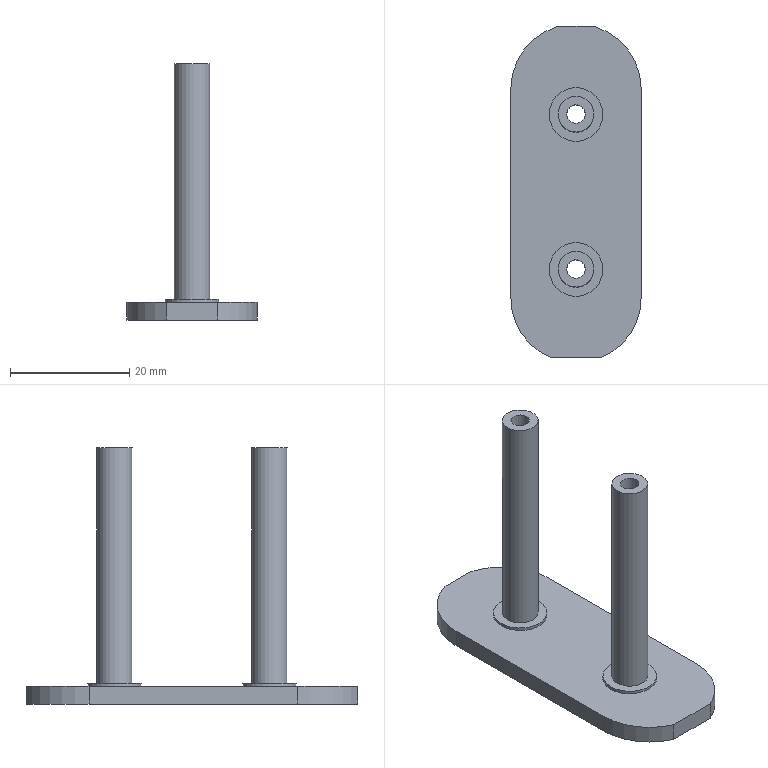Part | STEP file | Wytnij-wyci_gni_cie1 | 1 solid | 20 faces | box 21.875 x 55.54 x 43 mm | volume 5051 mm3 | cylinder 10 | plane 10 | commonest cylinder face diameters 21.875 x4 3.1 x2 6 x2 9 x2
STEP:
#1=CARTESIAN_POINT('',(0.,0.,0.));
#2=DIRECTION('',(0.,0.,1.));
#3=DIRECTION('',(1.,0.,0.));
#4=AXIS2_PLACEMENT_3D('',#1,#2,#3);
#5=CARTESIAN_POINT('',(-37.194,75.138,-134.798));
#6=VERTEX_POINT('',#5);
#7=CARTESIAN_POINT('',(-38.744,75.138,-134.798));
#8=DIRECTION('',(0.,0.,-1.));
#9=DIRECTION('',(1.,0.,0.));
#10=AXIS2_PLACEMENT_3D('',#7,#8,#9);
#11=CIRCLE('',#10,1.55);
#12=CARTESIAN_POINT('',(-38.744,75.138,-134.798));
#13=DIRECTION('',(0.,0.,1.));
#14=DIRECTION('',(1.,0.,0.));
#15=AXIS2_PLACEMENT_3D('',#12,#13,#14);
#16=CYLINDRICAL_SURFACE('',#15,1.55);
#17=CARTESIAN_POINT('',(6.283,0.));
#18=DIRECTION('',(-1.,0.));
#19=VECTOR('',#18,1.);
#20=LINE('',#17,#19);
#21=(GEOMETRIC_REPRESENTATION_CONTEXT(2)PARAMETRIC_REPRESENTATION_CONTEXT()REPRESENTATION_CONTEXT('',''));
#22=DEFINITIONAL_REPRESENTATION('',(#20),#21);
#23=PCURVE('',#16,#22);
#24=CARTESIAN_POINT('',(-38.744,88.138,-134.798));
#25=DIRECTION('',(0.,0.,1.));
#26=DIRECTION('',(1.,0.,0.));
#27=AXIS2_PLACEMENT_3D('',#24,#25,#26);
#28=PLANE('',#27);
#29=CARTESIAN_POINT('',(1.55,-13.));
#30=CARTESIAN_POINT('',(1.55,-15.685));
#31=CARTESIAN_POINT('',(-0.775,-14.342));
#32=CARTESIAN_POINT('',(-3.1,-13.));
#33=CARTESIAN_POINT('',(-0.775,-11.658));
#34=CARTESIAN_POINT('',(1.55,-10.315));
#35=CARTESIAN_POINT('',(1.55,-13.));
#36=(BOUNDED_CURVE()B_SPLINE_CURVE(2,(#29,#30,#31,#32,#33,#34,#35),.UNSPECIFIED.,.T.,.F.)B_SPLINE_CURVE_WITH_KNOTS((1,2,2,2,2,1),(-2.094,0.,2.094,4.189,6.283,8.378),.UNSPECIFIED.)CURVE()GEOMETRIC_REPRESENTATION_ITEM()RATIONAL_B_SPLINE_CURVE((1.,0.5,1.,0.5,1.,0.5,1.))REPRESENTATION_ITEM(''));
#37=(GEOMETRIC_REPRESENTATION_CONTEXT(2)PARAMETRIC_REPRESENTATION_CONTEXT()REPRESENTATION_CONTEXT('',''));
#38=DEFINITIONAL_REPRESENTATION('',(#36),#37);
#39=PCURVE('',#28,#38);
#40=SURFACE_CURVE('',#11,(#23,#39),.PCURVE_S1.);
#41=EDGE_CURVE('',#6,#6,#40,.T.);
#42=ORIENTED_EDGE('',*,*,#41,.F.);
#43=CARTESIAN_POINT('',(-37.194,75.138,-91.798));
#44=VERTEX_POINT('',#43);
#45=CARTESIAN_POINT('',(-37.194,75.138,-91.798));
#46=DIRECTION('',(0.,0.,-1.));
#47=VECTOR('',#46,1.);
#48=LINE('',#45,#47);
#49=CARTESIAN_POINT('',(6.283,43.));
#50=DIRECTION('',(0.,-1.));
#51=VECTOR('',#50,1.);
#52=LINE('',#49,#51);
#53=(GEOMETRIC_REPRESENTATION_CONTEXT(2)PARAMETRIC_REPRESENTATION_CONTEXT()REPRESENTATION_CONTEXT('',''));
#54=DEFINITIONAL_REPRESENTATION('',(#52),#53);
#55=PCURVE('',#16,#54);
#56=CARTESIAN_POINT('',(0.,43.));
#57=DIRECTION('',(0.,-1.));
#58=VECTOR('',#57,1.);
#59=LINE('',#56,#58);
#60=(GEOMETRIC_REPRESENTATION_CONTEXT(2)PARAMETRIC_REPRESENTATION_CONTEXT()REPRESENTATION_CONTEXT('',''));
#61=DEFINITIONAL_REPRESENTATION('',(#59),#60);
#62=PCURVE('',#16,#61);
#63=SEAM_CURVE('',#48,(#55,#62),.PCURVE_S1.);
#64=EDGE_CURVE('',#44,#6,#63,.T.);
#65=ORIENTED_EDGE('',*,*,#64,.F.);
#66=CARTESIAN_POINT('',(-38.744,75.138,-91.798));
#67=DIRECTION('',(0.,0.,-1.));
#68=DIRECTION('',(1.,0.,0.));
#69=AXIS2_PLACEMENT_3D('',#66,#67,#68);
#70=CIRCLE('',#69,1.55);
#71=CARTESIAN_POINT('',(6.283,43.));
#72=DIRECTION('',(-1.,0.));
#73=VECTOR('',#72,1.);
#74=LINE('',#71,#73);
#75=(GEOMETRIC_REPRESENTATION_CONTEXT(2)PARAMETRIC_REPRESENTATION_CONTEXT()REPRESENTATION_CONTEXT('',''));
#76=DEFINITIONAL_REPRESENTATION('',(#74),#75);
#77=PCURVE('',#16,#76);
#78=CARTESIAN_POINT('',(-38.744,75.138,-91.798));
#79=DIRECTION('',(0.,0.,1.));
#80=DIRECTION('',(1.,0.,0.));
#81=AXIS2_PLACEMENT_3D('',#78,#79,#80);
#82=PLANE('',#81);
#83=CARTESIAN_POINT('',(1.55,0.));
#84=CARTESIAN_POINT('',(1.55,-2.685));
#85=CARTESIAN_POINT('',(-0.775,-1.342));
#86=CARTESIAN_POINT('',(-3.1,0.));
#87=CARTESIAN_POINT('',(-0.775,1.342));
#88=CARTESIAN_POINT('',(1.55,2.685));
#89=CARTESIAN_POINT('',(1.55,0.));
#90=(BOUNDED_CURVE()B_SPLINE_CURVE(2,(#83,#84,#85,#86,#87,#88,#89),.UNSPECIFIED.,.T.,.F.)B_SPLINE_CURVE_WITH_KNOTS((1,2,2,2,2,1),(-2.094,0.,2.094,4.189,6.283,8.378),.UNSPECIFIED.)CURVE()GEOMETRIC_REPRESENTATION_ITEM()RATIONAL_B_SPLINE_CURVE((1.,0.5,1.,0.5,1.,0.5,1.))REPRESENTATION_ITEM(''));
#91=(GEOMETRIC_REPRESENTATION_CONTEXT(2)PARAMETRIC_REPRESENTATION_CONTEXT()REPRESENTATION_CONTEXT('',''));
#92=DEFINITIONAL_REPRESENTATION('',(#90),#91);
#93=PCURVE('',#82,#92);
#94=SURFACE_CURVE('',#70,(#77,#93),.PCURVE_S1.);
#95=EDGE_CURVE('',#44,#44,#94,.T.);
#96=ORIENTED_EDGE('',*,*,#95,.T.);
#97=ORIENTED_EDGE('',*,*,#64,.T.);
#98=EDGE_LOOP('',(#42,#65,#96,#97));
#99=FACE_BOUND('',#98,.F.);
#100=ADVANCED_FACE('',(#99),#16,.F.);
#101=CARTESIAN_POINT('',(-37.194,101.138,-134.798));
#102=VERTEX_POINT('',#101);
#103=CARTESIAN_POINT('',(-38.744,101.138,-134.798));
#104=DIRECTION('',(0.,0.,-1.));
#105=DIRECTION('',(1.,0.,0.));
#106=AXIS2_PLACEMENT_3D('',#103,#104,#105);
#107=CIRCLE('',#106,1.55);
#108=CARTESIAN_POINT('',(-38.744,101.138,-134.798));
#109=DIRECTION('',(0.,0.,1.));
#110=DIRECTION('',(1.,0.,0.));
#111=AXIS2_PLACEMENT_3D('',#108,#109,#110);
#112=CYLINDRICAL_SURFACE('',#111,1.55);
#113=CARTESIAN_POINT('',(6.283,0.));
#114=DIRECTION('',(-1.,0.));
#115=VECTOR('',#114,1.);
#116=LINE('',#113,#115);
#117=(GEOMETRIC_REPRESENTATION_CONTEXT(2)PARAMETRIC_REPRESENTATION_CONTEXT()REPRESENTATION_CONTEXT('',''));
#118=DEFINITIONAL_REPRESENTATION('',(#116),#117);
#119=PCURVE('',#112,#118);
#120=CARTESIAN_POINT('',(1.55,13.));
#121=CARTESIAN_POINT('',(1.55,10.315));
#122=CARTESIAN_POINT('',(-0.775,11.658));
#123=CARTESIAN_POINT('',(-3.1,13.));
#124=CARTESIAN_POINT('',(-0.775,14.342));
#125=CARTESIAN_POINT('',(1.55,15.685));
#126=CARTESIAN_POINT('',(1.55,13.));
#127=(BOUNDED_CURVE()B_SPLINE_CURVE(2,(#120,#121,#122,#123,#124,#125,#126),.UNSPECIFIED.,.T.,.F.)B_SPLINE_CURVE_WITH_KNOTS((1,2,2,2,2,1),(-2.094,0.,2.094,4.189,6.283,8.378),.UNSPECIFIED.)CURVE()GEOMETRIC_REPRESENTATION_ITEM()RATIONAL_B_SPLINE_CURVE((1.,0.5,1.,0.5,1.,0.5,1.))REPRESENTATION_ITEM(''));
#128=(GEOMETRIC_REPRESENTATION_CONTEXT(2)PARAMETRIC_REPRESENTATION_CONTEXT()REPRESENTATION_CONTEXT('',''));
#129=DEFINITIONAL_REPRESENTATION('',(#127),#128);
#130=PCURVE('',#28,#129);
#131=SURFACE_CURVE('',#107,(#119,#130),.PCURVE_S1.);
#132=EDGE_CURVE('',#102,#102,#131,.T.);
#133=ORIENTED_EDGE('',*,*,#132,.F.);
#134=CARTESIAN_POINT('',(-37.194,101.138,-91.798));
#135=VERTEX_POINT('',#134);
#136=CARTESIAN_POINT('',(-37.194,101.138,-91.798));
#137=DIRECTION('',(0.,0.,-1.));
#138=VECTOR('',#137,1.);
#139=LINE('',#136,#138);
#140=CARTESIAN_POINT('',(6.283,43.));
#141=DIRECTION('',(0.,-1.));
#142=VECTOR('',#141,1.);
#143=LINE('',#140,#142);
#144=(GEOMETRIC_REPRESENTATION_CONTEXT(2)PARAMETRIC_REPRESENTATION_CONTEXT()REPRESENTATION_CONTEXT('',''));
#145=DEFINITIONAL_REPRESENTATION('',(#143),#144);
#146=PCURVE('',#112,#145);
#147=CARTESIAN_POINT('',(0.,43.));
#148=DIRECTION('',(0.,-1.));
#149=VECTOR('',#148,1.);
#150=LINE('',#147,#149);
#151=(GEOMETRIC_REPRESENTATION_CONTEXT(2)PARAMETRIC_REPRESENTATION_CONTEXT()REPRESENTATION_CONTEXT('',''));
#152=DEFINITIONAL_REPRESENTATION('',(#150),#151);
#153=PCURVE('',#112,#152);
#154=SEAM_CURVE('',#139,(#146,#153),.PCURVE_S1.);
#155=EDGE_CURVE('',#135,#102,#154,.T.);
#156=ORIENTED_EDGE('',*,*,#155,.F.);
#157=CARTESIAN_POINT('',(-38.744,101.138,-91.798));
#158=DIRECTION('',(0.,0.,-1.));
#159=DIRECTION('',(1.,0.,0.));
#160=AXIS2_PLACEMENT_3D('',#157,#158,#159);
#161=CIRCLE('',#160,1.55);
#162=CARTESIAN_POINT('',(6.283,43.));
#163=DIRECTION('',(-1.,0.));
#164=VECTOR('',#163,1.);
#165=LINE('',#162,#164);
#166=(GEOMETRIC_REPRESENTATION_CONTEXT(2)PARAMETRIC_REPRESENTATION_CONTEXT()REPRESENTATION_CONTEXT('',''));
#167=DEFINITIONAL_REPRESENTATION('',(#165),#166);
#168=PCURVE('',#112,#167);
#169=CARTESIAN_POINT('',(-38.744,101.138,-91.798));
#170=DIRECTION('',(0.,0.,1.));
#171=DIRECTION('',(1.,0.,0.));
#172=AXIS2_PLACEMENT_3D('',#169,#170,#171);
#173=PLANE('',#172);
#174=CARTESIAN_POINT('',(1.55,0.));
#175=CARTESIAN_POINT('',(1.55,-2.685));
#176=CARTESIAN_POINT('',(-0.775,-1.342));
#177=CARTESIAN_POINT('',(-3.1,0.));
#178=CARTESIAN_POINT('',(-0.775,1.342));
#179=CARTESIAN_POINT('',(1.55,2.685));
#180=CARTESIAN_POINT('',(1.55,0.));
#181=(BOUNDED_CURVE()B_SPLINE_CURVE(2,(#174,#175,#176,#177,#178,#179,#180),.UNSPECIFIED.,.T.,.F.)B_SPLINE_CURVE_WITH_KNOTS((1,2,2,2,2,1),(-2.094,0.,2.094,4.189,6.283,8.378),.UNSPECIFIED.)CURVE()GEOMETRIC_REPRESENTATION_ITEM()RATIONAL_B_SPLINE_CURVE((1.,0.5,1.,0.5,1.,0.5,1.))REPRESENTATION_ITEM(''));
#182=(GEOMETRIC_REPRESENTATION_CONTEXT(2)PARAMETRIC_REPRESENTATION_CONTEXT()REPRESENTATION_CONTEXT('',''));
#183=DEFINITIONAL_REPRESENTATION('',(#181),#182);
#184=PCURVE('',#173,#183);
#185=SURFACE_CURVE('',#161,(#168,#184),.PCURVE_S1.);
#186=EDGE_CURVE('',#135,#135,#185,.T.);
#187=ORIENTED_EDGE('',*,*,#186,.T.);
#188=ORIENTED_EDGE('',*,*,#155,.T.);
#189=EDGE_LOOP('',(#133,#156,#187,#188));
#190=FACE_BOUND('',#189,.F.);
#191=ADVANCED_FACE('',(#190),#112,.F.);
#192=CARTESIAN_POINT('',(-41.744,75.138,-131.298));
#193=VERTEX_POINT('',#192);
#194=CARTESIAN_POINT('',(-41.744,75.138,-91.798));
#195=VERTEX_POINT('',#194);
#196=CARTESIAN_POINT('',(-41.744,75.138,-131.298));
#197=DIRECTION('',(0.,0.,1.));
#198=VECTOR('',#197,1.);
#199=LINE('',#196,#198);
#200=CARTESIAN_POINT('',(-38.744,75.138,-91.798));
#201=DIRECTION('',(0.,0.,-1.));
#202=DIRECTION('',(-1.,0.,0.));
#203=AXIS2_PLACEMENT_3D('',#200,#201,#202);
#204=CYLINDRICAL_SURFACE('',#203,3.);
#205=CARTESIAN_POINT('',(0.,39.5));
#206=DIRECTION('',(0.,-1.));
#207=VECTOR('',#206,1.);
#208=LINE('',#205,#207);
#209=(GEOMETRIC_REPRESENTATION_CONTEXT(2)PARAMETRIC_REPRESENTATION_CONTEXT()REPRESENTATION_CONTEXT('',''));
#210=DEFINITIONAL_REPRESENTATION('',(#208),#209);
#211=PCURVE('',#204,#210);
#212=CARTESIAN_POINT('',(6.283,39.5));
#213=DIRECTION('',(0.,-1.));
#214=VECTOR('',#213,1.);
#215=LINE('',#212,#214);
#216=(GEOMETRIC_REPRESENTATION_CONTEXT(2)PARAMETRIC_REPRESENTATION_CONTEXT()REPRESENTATION_CONTEXT('',''));
#217=DEFINITIONAL_REPRESENTATION('',(#215),#216);
#218=PCURVE('',#204,#217);
#219=SEAM_CURVE('',#199,(#211,#218),.PCURVE_S1.);
#220=EDGE_CURVE('',#193,#195,#219,.T.);
#221=ORIENTED_EDGE('',*,*,#220,.T.);
#222=CARTESIAN_POINT('',(-38.744,75.138,-91.798));
#223=DIRECTION('',(0.,0.,1.));
#224=DIRECTION('',(-1.,0.,0.));
#225=AXIS2_PLACEMENT_3D('',#222,#223,#224);
#226=CIRCLE('',#225,3.);
#227=CARTESIAN_POINT('',(6.283,0.));
#228=DIRECTION('',(-1.,0.));
#229=VECTOR('',#228,1.);
#230=LINE('',#227,#229);
#231=(GEOMETRIC_REPRESENTATION_CONTEXT(2)PARAMETRIC_REPRESENTATION_CONTEXT()REPRESENTATION_CONTEXT('',''));
#232=DEFINITIONAL_REPRESENTATION('',(#230),#231);
#233=PCURVE('',#204,#232);
#234=CARTESIAN_POINT('',(0.,0.));
#235=DIRECTION('',(-1.,0.));
#236=AXIS2_PLACEMENT_2D('',#234,#235);
#237=CIRCLE('',#236,3.);
#238=(GEOMETRIC_REPRESENTATION_CONTEXT(2)PARAMETRIC_REPRESENTATION_CONTEXT()REPRESENTATION_CONTEXT('',''));
#239=DEFINITIONAL_REPRESENTATION('',(#237),#238);
#240=PCURVE('',#82,#239);
#241=SURFACE_CURVE('',#226,(#233,#240),.PCURVE_S1.);
#242=EDGE_CURVE('',#195,#195,#241,.T.);
#243=ORIENTED_EDGE('',*,*,#242,.F.);
#244=ORIENTED_EDGE('',*,*,#220,.F.);
#245=CARTESIAN_POINT('',(-38.744,75.138,-131.298));
#246=DIRECTION('',(0.,0.,1.));
#247=DIRECTION('',(-1.,0.,0.));
#248=AXIS2_PLACEMENT_3D('',#245,#246,#247);
#249=CIRCLE('',#248,3.);
#250=CARTESIAN_POINT('',(6.283,39.5));
#251=DIRECTION('',(-1.,0.));
#252=VECTOR('',#251,1.);
#253=LINE('',#250,#252);
#254=(GEOMETRIC_REPRESENTATION_CONTEXT(2)PARAMETRIC_REPRESENTATION_CONTEXT()REPRESENTATION_CONTEXT('',''));
#255=DEFINITIONAL_REPRESENTATION('',(#253),#254);
#256=PCURVE('',#204,#255);
#257=CARTESIAN_POINT('',(-38.744,75.138,-131.298));
#258=DIRECTION('',(0.,0.,1.));
#259=DIRECTION('',(1.,0.,0.));
#260=AXIS2_PLACEMENT_3D('',#257,#258,#259);
#261=PLANE('',#260);
#262=CARTESIAN_POINT('',(0.,0.));
#263=DIRECTION('',(-1.,0.));
#264=AXIS2_PLACEMENT_2D('',#262,#263);
#265=CIRCLE('',#264,3.);
#266=(GEOMETRIC_REPRESENTATION_CONTEXT(2)PARAMETRIC_REPRESENTATION_CONTEXT()REPRESENTATION_CONTEXT('',''));
#267=DEFINITIONAL_REPRESENTATION('',(#265),#266);
#268=PCURVE('',#261,#267);
#269=SURFACE_CURVE('',#249,(#256,#268),.PCURVE_S1.);
#270=EDGE_CURVE('',#193,#193,#269,.T.);
#271=ORIENTED_EDGE('',*,*,#270,.T.);
#272=EDGE_LOOP('',(#221,#243,#244,#271));
#273=FACE_BOUND('',#272,.T.);
#274=ADVANCED_FACE('',(#273),#204,.T.);
#275=CARTESIAN_POINT('',(-41.744,101.138,-131.298));
#276=VERTEX_POINT('',#275);
#277=CARTESIAN_POINT('',(-41.744,101.138,-91.798));
#278=VERTEX_POINT('',#277);
#279=CARTESIAN_POINT('',(-41.744,101.138,-131.298));
#280=DIRECTION('',(0.,0.,1.));
#281=VECTOR('',#280,1.);
#282=LINE('',#279,#281);
#283=CARTESIAN_POINT('',(-38.744,101.138,-91.798));
#284=DIRECTION('',(0.,0.,-1.));
#285=DIRECTION('',(-1.,0.,0.));
#286=AXIS2_PLACEMENT_3D('',#283,#284,#285);
#287=CYLINDRICAL_SURFACE('',#286,3.);
#288=CARTESIAN_POINT('',(0.,39.5));
#289=DIRECTION('',(0.,-1.));
#290=VECTOR('',#289,1.);
#291=LINE('',#288,#290);
#292=(GEOMETRIC_REPRESENTATION_CONTEXT(2)PARAMETRIC_REPRESENTATION_CONTEXT()REPRESENTATION_CONTEXT('',''));
#293=DEFINITIONAL_REPRESENTATION('',(#291),#292);
#294=PCURVE('',#287,#293);
#295=CARTESIAN_POINT('',(6.283,39.5));
#296=DIRECTION('',(0.,-1.));
#297=VECTOR('',#296,1.);
#298=LINE('',#295,#297);
#299=(GEOMETRIC_REPRESENTATION_CONTEXT(2)PARAMETRIC_REPRESENTATION_CONTEXT()REPRESENTATION_CONTEXT('',''));
#300=DEFINITIONAL_REPRESENTATION('',(#298),#299);
#301=PCURVE('',#287,#300);
#302=SEAM_CURVE('',#282,(#294,#301),.PCURVE_S1.);
#303=EDGE_CURVE('',#276,#278,#302,.T.);
#304=ORIENTED_EDGE('',*,*,#303,.T.);
#305=CARTESIAN_POINT('',(-38.744,101.138,-91.798));
#306=DIRECTION('',(0.,0.,1.));
#307=DIRECTION('',(-1.,0.,0.));
#308=AXIS2_PLACEMENT_3D('',#305,#306,#307);
#309=CIRCLE('',#308,3.);
#310=CARTESIAN_POINT('',(6.283,0.));
#311=DIRECTION('',(-1.,0.));
#312=VECTOR('',#311,1.);
#313=LINE('',#310,#312);
#314=(GEOMETRIC_REPRESENTATION_CONTEXT(2)PARAMETRIC_REPRESENTATION_CONTEXT()REPRESENTATION_CONTEXT('',''));
#315=DEFINITIONAL_REPRESENTATION('',(#313),#314);
#316=PCURVE('',#287,#315);
#317=CARTESIAN_POINT('',(0.,0.));
#318=DIRECTION('',(-1.,0.));
#319=AXIS2_PLACEMENT_2D('',#317,#318);
#320=CIRCLE('',#319,3.);
#321=(GEOMETRIC_REPRESENTATION_CONTEXT(2)PARAMETRIC_REPRESENTATION_CONTEXT()REPRESENTATION_CONTEXT('',''));
#322=DEFINITIONAL_REPRESENTATION('',(#320),#321);
#323=PCURVE('',#173,#322);
#324=SURFACE_CURVE('',#309,(#316,#323),.PCURVE_S1.);
#325=EDGE_CURVE('',#278,#278,#324,.T.);
#326=ORIENTED_EDGE('',*,*,#325,.F.);
#327=ORIENTED_EDGE('',*,*,#303,.F.);
#328=CARTESIAN_POINT('',(-38.744,101.138,-131.298));
#329=DIRECTION('',(0.,0.,1.));
#330=DIRECTION('',(-1.,0.,0.));
#331=AXIS2_PLACEMENT_3D('',#328,#329,#330);
#332=CIRCLE('',#331,3.);
#333=CARTESIAN_POINT('',(6.283,39.5));
#334=DIRECTION('',(-1.,0.));
#335=VECTOR('',#334,1.);
#336=LINE('',#333,#335);
#337=(GEOMETRIC_REPRESENTATION_CONTEXT(2)PARAMETRIC_REPRESENTATION_CONTEXT()REPRESENTATION_CONTEXT('',''));
#338=DEFINITIONAL_REPRESENTATION('',(#336),#337);
#339=PCURVE('',#287,#338);
#340=CARTESIAN_POINT('',(-38.744,101.138,-131.298));
#341=DIRECTION('',(0.,0.,1.));
#342=DIRECTION('',(1.,0.,0.));
#343=AXIS2_PLACEMENT_3D('',#340,#341,#342);
#344=PLANE('',#343);
#345=CARTESIAN_POINT('',(0.,0.));
#346=DIRECTION('',(-1.,0.));
#347=AXIS2_PLACEMENT_2D('',#345,#346);
#348=CIRCLE('',#347,3.);
#349=(GEOMETRIC_REPRESENTATION_CONTEXT(2)PARAMETRIC_REPRESENTATION_CONTEXT()REPRESENTATION_CONTEXT('',''));
#350=DEFINITIONAL_REPRESENTATION('',(#348),#349);
#351=PCURVE('',#344,#350);
#352=SURFACE_CURVE('',#332,(#339,#351),.PCURVE_S1.);
#353=EDGE_CURVE('',#276,#276,#352,.T.);
#354=ORIENTED_EDGE('',*,*,#353,.T.);
#355=EDGE_LOOP('',(#304,#326,#327,#354));
#356=FACE_BOUND('',#355,.T.);
#357=ADVANCED_FACE('',(#356),#287,.T.);
#358=CARTESIAN_POINT('',(-43.244,101.138,-131.798));
#359=VERTEX_POINT('',#358);
#360=CARTESIAN_POINT('',(-43.244,101.138,-131.298));
#361=VERTEX_POINT('',#360);
#362=CARTESIAN_POINT('',(-43.244,101.138,-131.798));
#363=DIRECTION('',(0.,0.,1.));
#364=VECTOR('',#363,1.);
#365=LINE('',#362,#364);
#366=CARTESIAN_POINT('',(-38.744,101.138,-131.298));
#367=DIRECTION('',(0.,0.,-1.));
#368=DIRECTION('',(-1.,0.,0.));
#369=AXIS2_PLACEMENT_3D('',#366,#367,#368);
#370=CYLINDRICAL_SURFACE('',#369,4.5);
#371=CARTESIAN_POINT('',(0.,0.5));
#372=DIRECTION('',(0.,-1.));
#373=VECTOR('',#372,1.);
#374=LINE('',#371,#373);
#375=(GEOMETRIC_REPRESENTATION_CONTEXT(2)PARAMETRIC_REPRESENTATION_CONTEXT()REPRESENTATION_CONTEXT('',''));
#376=DEFINITIONAL_REPRESENTATION('',(#374),#375);
#377=PCURVE('',#370,#376);
#378=CARTESIAN_POINT('',(6.283,0.5));
#379=DIRECTION('',(0.,-1.));
#380=VECTOR('',#379,1.);
#381=LINE('',#378,#380);
#382=(GEOMETRIC_REPRESENTATION_CONTEXT(2)PARAMETRIC_REPRESENTATION_CONTEXT()REPRESENTATION_CONTEXT('',''));
#383=DEFINITIONAL_REPRESENTATION('',(#381),#382);
#384=PCURVE('',#370,#383);
#385=SEAM_CURVE('',#365,(#377,#384),.PCURVE_S1.);
#386=EDGE_CURVE('',#359,#361,#385,.T.);
#387=ORIENTED_EDGE('',*,*,#386,.T.);
#388=CARTESIAN_POINT('',(-38.744,101.138,-131.298));
#389=DIRECTION('',(0.,0.,-1.));
#390=DIRECTION('',(-1.,0.,0.));
#391=AXIS2_PLACEMENT_3D('',#388,#389,#390);
#392=CIRCLE('',#391,4.5);
#393=CARTESIAN_POINT('',(0.,0.));
#394=DIRECTION('',(1.,0.));
#395=VECTOR('',#394,1.);
#396=LINE('',#393,#395);
#397=(GEOMETRIC_REPRESENTATION_CONTEXT(2)PARAMETRIC_REPRESENTATION_CONTEXT()REPRESENTATION_CONTEXT('',''));
#398=DEFINITIONAL_REPRESENTATION('',(#396),#397);
#399=PCURVE('',#370,#398);
#400=CARTESIAN_POINT('',(-4.5,0.));
#401=CARTESIAN_POINT('',(-4.5,7.794));
#402=CARTESIAN_POINT('',(2.25,3.897));
#403=CARTESIAN_POINT('',(9.,0.));
#404=CARTESIAN_POINT('',(2.25,-3.897));
#405=CARTESIAN_POINT('',(-4.5,-7.794));
#406=CARTESIAN_POINT('',(-4.5,0.));
#407=(BOUNDED_CURVE()B_SPLINE_CURVE(2,(#400,#401,#402,#403,#404,#405,#406),.UNSPECIFIED.,.T.,.F.)B_SPLINE_CURVE_WITH_KNOTS((1,2,2,2,2,1),(-2.094,0.,2.094,4.189,6.283,8.378),.UNSPECIFIED.)CURVE()GEOMETRIC_REPRESENTATION_ITEM()RATIONAL_B_SPLINE_CURVE((1.,0.5,1.,0.5,1.,0.5,1.))REPRESENTATION_ITEM(''));
#408=(GEOMETRIC_REPRESENTATION_CONTEXT(2)PARAMETRIC_REPRESENTATION_CONTEXT()REPRESENTATION_CONTEXT('',''));
#409=DEFINITIONAL_REPRESENTATION('',(#407),#408);
#410=PCURVE('',#344,#409);
#411=SURFACE_CURVE('',#392,(#399,#410),.PCURVE_S1.);
#412=EDGE_CURVE('',#361,#361,#411,.T.);
#413=ORIENTED_EDGE('',*,*,#412,.T.);
#414=ORIENTED_EDGE('',*,*,#386,.F.);
#415=CARTESIAN_POINT('',(-38.744,101.138,-131.798));
#416=DIRECTION('',(0.,0.,-1.));
#417=DIRECTION('',(-1.,0.,0.));
#418=AXIS2_PLACEMENT_3D('',#415,#416,#417);
#419=CIRCLE('',#418,4.5);
#420=CARTESIAN_POINT('',(0.,0.5));
#421=DIRECTION('',(1.,0.));
#422=VECTOR('',#421,1.);
#423=LINE('',#420,#422);
#424=(GEOMETRIC_REPRESENTATION_CONTEXT(2)PARAMETRIC_REPRESENTATION_CONTEXT()REPRESENTATION_CONTEXT('',''));
#425=DEFINITIONAL_REPRESENTATION('',(#423),#424);
#426=PCURVE('',#370,#425);
#427=CARTESIAN_POINT('',(-38.744,88.138,-131.798));
#428=DIRECTION('',(0.,0.,1.));
#429=DIRECTION('',(1.,0.,0.));
#430=AXIS2_PLACEMENT_3D('',#427,#428,#429);
#431=PLANE('',#430);
#432=CARTESIAN_POINT('',(-4.5,13.));
#433=CARTESIAN_POINT('',(-4.5,20.794));
#434=CARTESIAN_POINT('',(2.25,16.897));
#435=CARTESIAN_POINT('',(9.,13.));
#436=CARTESIAN_POINT('',(2.25,9.103));
#437=CARTESIAN_POINT('',(-4.5,5.206));
#438=CARTESIAN_POINT('',(-4.5,13.));
#439=(BOUNDED_CURVE()B_SPLINE_CURVE(2,(#432,#433,#434,#435,#436,#437,#438),.UNSPECIFIED.,.T.,.F.)B_SPLINE_CURVE_WITH_KNOTS((1,2,2,2,2,1),(-2.094,0.,2.094,4.189,6.283,8.378),.UNSPECIFIED.)CURVE()GEOMETRIC_REPRESENTATION_ITEM()RATIONAL_B_SPLINE_CURVE((1.,0.5,1.,0.5,1.,0.5,1.))REPRESENTATION_ITEM(''));
#440=(GEOMETRIC_REPRESENTATION_CONTEXT(2)PARAMETRIC_REPRESENTATION_CONTEXT()REPRESENTATION_CONTEXT('',''));
#441=DEFINITIONAL_REPRESENTATION('',(#439),#440);
#442=PCURVE('',#431,#441);
#443=SURFACE_CURVE('',#419,(#426,#442),.PCURVE_S1.);
#444=EDGE_CURVE('',#359,#359,#443,.T.);
#445=ORIENTED_EDGE('',*,*,#444,.F.);
#446=EDGE_LOOP('',(#387,#413,#414,#445));
#447=FACE_BOUND('',#446,.T.);
#448=ADVANCED_FACE('',(#447),#370,.T.);
#449=CARTESIAN_POINT('',(-43.244,75.138,-131.798));
#450=VERTEX_POINT('',#449);
#451=CARTESIAN_POINT('',(-43.244,75.138,-131.298));
#452=VERTEX_POINT('',#451);
#453=CARTESIAN_POINT('',(-43.244,75.138,-131.798));
#454=DIRECTION('',(0.,0.,1.));
#455=VECTOR('',#454,1.);
#456=LINE('',#453,#455);
#457=CARTESIAN_POINT('',(-38.744,75.138,-131.298));
#458=DIRECTION('',(0.,0.,-1.));
#459=DIRECTION('',(-1.,0.,0.));
#460=AXIS2_PLACEMENT_3D('',#457,#458,#459);
#461=CYLINDRICAL_SURFACE('',#460,4.5);
#462=CARTESIAN_POINT('',(0.,0.5));
#463=DIRECTION('',(0.,-1.));
#464=VECTOR('',#463,1.);
#465=LINE('',#462,#464);
#466=(GEOMETRIC_REPRESENTATION_CONTEXT(2)PARAMETRIC_REPRESENTATION_CONTEXT()REPRESENTATION_CONTEXT('',''));
#467=DEFINITIONAL_REPRESENTATION('',(#465),#466);
#468=PCURVE('',#461,#467);
#469=CARTESIAN_POINT('',(6.283,0.5));
#470=DIRECTION('',(0.,-1.));
#471=VECTOR('',#470,1.);
#472=LINE('',#469,#471);
#473=(GEOMETRIC_REPRESENTATION_CONTEXT(2)PARAMETRIC_REPRESENTATION_CONTEXT()REPRESENTATION_CONTEXT('',''));
#474=DEFINITIONAL_REPRESENTATION('',(#472),#473);
#475=PCURVE('',#461,#474);
#476=SEAM_CURVE('',#456,(#468,#475),.PCURVE_S1.);
#477=EDGE_CURVE('',#450,#452,#476,.T.);
#478=ORIENTED_EDGE('',*,*,#477,.T.);
#479=CARTESIAN_POINT('',(-38.744,75.138,-131.298));
#480=DIRECTION('',(0.,0.,-1.));
#481=DIRECTION('',(-1.,0.,0.));
#482=AXIS2_PLACEMENT_3D('',#479,#480,#481);
#483=CIRCLE('',#482,4.5);
#484=CARTESIAN_POINT('',(0.,0.));
#485=DIRECTION('',(1.,0.));
#486=VECTOR('',#485,1.);
#487=LINE('',#484,#486);
#488=(GEOMETRIC_REPRESENTATION_CONTEXT(2)PARAMETRIC_REPRESENTATION_CONTEXT()REPRESENTATION_CONTEXT('',''));
#489=DEFINITIONAL_REPRESENTATION('',(#487),#488);
#490=PCURVE('',#461,#489);
#491=CARTESIAN_POINT('',(-4.5,0.));
#492=CARTESIAN_POINT('',(-4.5,7.794));
#493=CARTESIAN_POINT('',(2.25,3.897));
#494=CARTESIAN_POINT('',(9.,0.));
#495=CARTESIAN_POINT('',(2.25,-3.897));
#496=CARTESIAN_POINT('',(-4.5,-7.794));
#497=CARTESIAN_POINT('',(-4.5,0.));
#498=(BOUNDED_CURVE()B_SPLINE_CURVE(2,(#491,#492,#493,#494,#495,#496,#497),.UNSPECIFIED.,.T.,.F.)B_SPLINE_CURVE_WITH_KNOTS((1,2,2,2,2,1),(-2.094,0.,2.094,4.189,6.283,8.378),.UNSPECIFIED.)CURVE()GEOMETRIC_REPRESENTATION_ITEM()RATIONAL_B_SPLINE_CURVE((1.,0.5,1.,0.5,1.,0.5,1.))REPRESENTATION_ITEM(''));
#499=(GEOMETRIC_REPRESENTATION_CONTEXT(2)PARAMETRIC_REPRESENTATION_CONTEXT()REPRESENTATION_CONTEXT('',''));
#500=DEFINITIONAL_REPRESENTATION('',(#498),#499);
#501=PCURVE('',#261,#500);
#502=SURFACE_CURVE('',#483,(#490,#501),.PCURVE_S1.);
#503=EDGE_CURVE('',#452,#452,#502,.T.);
#504=ORIENTED_EDGE('',*,*,#503,.T.);
#505=ORIENTED_EDGE('',*,*,#477,.F.);
#506=CARTESIAN_POINT('',(-38.744,75.138,-131.798));
#507=DIRECTION('',(0.,0.,-1.));
#508=DIRECTION('',(-1.,0.,0.));
#509=AXIS2_PLACEMENT_3D('',#506,#507,#508);
#510=CIRCLE('',#509,4.5);
#511=CARTESIAN_POINT('',(0.,0.5));
#512=DIRECTION('',(1.,0.));
#513=VECTOR('',#512,1.);
#514=LINE('',#511,#513);
#515=(GEOMETRIC_REPRESENTATION_CONTEXT(2)PARAMETRIC_REPRESENTATION_CONTEXT()REPRESENTATION_CONTEXT('',''));
#516=DEFINITIONAL_REPRESENTATION('',(#514),#515);
#517=PCURVE('',#461,#516);
#518=CARTESIAN_POINT('',(-4.5,-13.));
#519=CARTESIAN_POINT('',(-4.5,-5.206));
#520=CARTESIAN_POINT('',(2.25,-9.103));
#521=CARTESIAN_POINT('',(9.,-13.));
#522=CARTESIAN_POINT('',(2.25,-16.897));
#523=CARTESIAN_POINT('',(-4.5,-20.794));
#524=CARTESIAN_POINT('',(-4.5,-13.));
#525=(BOUNDED_CURVE()B_SPLINE_CURVE(2,(#518,#519,#520,#521,#522,#523,#524),.UNSPECIFIED.,.T.,.F.)B_SPLINE_CURVE_WITH_KNOTS((1,2,2,2,2,1),(-2.094,0.,2.094,4.189,6.283,8.378),.UNSPECIFIED.)CURVE()GEOMETRIC_REPRESENTATION_ITEM()RATIONAL_B_SPLINE_CURVE((1.,0.5,1.,0.5,1.,0.5,1.))REPRESENTATION_ITEM(''));
#526=(GEOMETRIC_REPRESENTATION_CONTEXT(2)PARAMETRIC_REPRESENTATION_CONTEXT()REPRESENTATION_CONTEXT('',''));
#527=DEFINITIONAL_REPRESENTATION('',(#525),#526);
#528=PCURVE('',#431,#527);
#529=SURFACE_CURVE('',#510,(#517,#528),.PCURVE_S1.);
#530=EDGE_CURVE('',#450,#450,#529,.T.);
#531=ORIENTED_EDGE('',*,*,#530,.F.);
#532=EDGE_LOOP('',(#478,#504,#505,#531));
#533=FACE_BOUND('',#532,.T.);
#534=ADVANCED_FACE('',(#533),#461,.T.);
#535=ORIENTED_EDGE('',*,*,#41,.F.);
#536=EDGE_LOOP('',(#535));
#537=FACE_BOUND('',#536,.T.);
#538=ORIENTED_EDGE('',*,*,#132,.F.);
#539=EDGE_LOOP('',(#538));
#540=FACE_BOUND('',#539,.T.);
#541=CARTESIAN_POINT('',(-27.807,70.408,-134.798));
#542=VERTEX_POINT('',#541);
#543=CARTESIAN_POINT('',(-27.807,105.408,-134.798));
#544=VERTEX_POINT('',#543);
#545=CARTESIAN_POINT('',(-27.807,70.408,-134.798));
#546=DIRECTION('',(0.,1.,0.));
#547=VECTOR('',#546,1.);
#548=LINE('',#545,#547);
#549=CARTESIAN_POINT('',(10.938,-17.73));
#550=DIRECTION('',(0.,1.));
#551=VECTOR('',#550,1.);
#552=LINE('',#549,#551);
#553=(GEOMETRIC_REPRESENTATION_CONTEXT(2)PARAMETRIC_REPRESENTATION_CONTEXT()REPRESENTATION_CONTEXT('',''));
#554=DEFINITIONAL_REPRESENTATION('',(#552),#553);
#555=PCURVE('',#28,#554);
#556=CARTESIAN_POINT('',(-27.807,87.908,-133.298));
#557=DIRECTION('',(-1.,0.,0.));
#558=DIRECTION('',(0.,-1.,0.));
#559=AXIS2_PLACEMENT_3D('',#556,#557,#558);
#560=PLANE('',#559);
#561=CARTESIAN_POINT('',(17.5,-1.5));
#562=DIRECTION('',(-1.,0.));
#563=VECTOR('',#562,1.);
#564=LINE('',#561,#563);
#565=(GEOMETRIC_REPRESENTATION_CONTEXT(2)PARAMETRIC_REPRESENTATION_CONTEXT()REPRESENTATION_CONTEXT('',''));
#566=DEFINITIONAL_REPRESENTATION('',(#564),#565);
#567=PCURVE('',#560,#566);
#568=SURFACE_CURVE('',#548,(#555,#567),.PCURVE_S1.);
#569=EDGE_CURVE('',#542,#544,#568,.T.);
#570=ORIENTED_EDGE('',*,*,#569,.F.);
#571=CARTESIAN_POINT('',(-34.405,60.368,-134.798));
#572=VERTEX_POINT('',#571);
#573=CARTESIAN_POINT('',(-38.744,70.408,-134.798));
#574=DIRECTION('',(0.,0.,1.));
#575=DIRECTION('',(-1.,0.,0.));
#576=AXIS2_PLACEMENT_3D('',#573,#574,#575);
#577=CIRCLE('',#576,10.938);
#578=CARTESIAN_POINT('',(0.,-17.73));
#579=DIRECTION('',(-1.,0.));
#580=AXIS2_PLACEMENT_2D('',#578,#579);
#581=CIRCLE('',#580,10.938);
#582=(GEOMETRIC_REPRESENTATION_CONTEXT(2)PARAMETRIC_REPRESENTATION_CONTEXT()REPRESENTATION_CONTEXT('',''));
#583=DEFINITIONAL_REPRESENTATION('',(#581),#582);
#584=PCURVE('',#28,#583);
#585=CARTESIAN_POINT('',(-38.744,70.408,-131.798));
#586=DIRECTION('',(0.,0.,-1.));
#587=DIRECTION('',(-1.,0.,0.));
#588=AXIS2_PLACEMENT_3D('',#585,#586,#587);
#589=CYLINDRICAL_SURFACE('',#588,10.938);
#590=CARTESIAN_POINT('',(6.283,3.));
#591=DIRECTION('',(-1.,0.));
#592=VECTOR('',#591,1.);
#593=LINE('',#590,#592);
#594=(GEOMETRIC_REPRESENTATION_CONTEXT(2)PARAMETRIC_REPRESENTATION_CONTEXT()REPRESENTATION_CONTEXT('',''));
#595=DEFINITIONAL_REPRESENTATION('',(#593),#594);
#596=PCURVE('',#589,#595);
#597=SURFACE_CURVE('',#577,(#584,#596),.PCURVE_S1.);
#598=EDGE_CURVE('',#572,#542,#597,.T.);
#599=ORIENTED_EDGE('',*,*,#598,.F.);
#600=CARTESIAN_POINT('',(-43.083,60.368,-134.798));
#601=VERTEX_POINT('',#600);
#602=CARTESIAN_POINT('',(-43.083,60.368,-134.798));
#603=DIRECTION('',(1.,0.,0.));
#604=VECTOR('',#603,1.);
#605=LINE('',#602,#604);
#606=CARTESIAN_POINT('',(-4.339,-27.77));
#607=DIRECTION('',(1.,0.));
#608=VECTOR('',#607,1.);
#609=LINE('',#606,#608);
#610=(GEOMETRIC_REPRESENTATION_CONTEXT(2)PARAMETRIC_REPRESENTATION_CONTEXT()REPRESENTATION_CONTEXT('',''));
#611=DEFINITIONAL_REPRESENTATION('',(#609),#610);
#612=PCURVE('',#28,#611);
#613=CARTESIAN_POINT('',(-38.744,60.368,-133.298));
#614=DIRECTION('',(0.,1.,0.));
#615=DIRECTION('',(-1.,0.,0.));
#616=AXIS2_PLACEMENT_3D('',#613,#614,#615);
#617=PLANE('',#616);
#618=CARTESIAN_POINT('',(4.339,-1.5));
#619=DIRECTION('',(-1.,0.));
#620=VECTOR('',#619,1.);
#621=LINE('',#618,#620);
#622=(GEOMETRIC_REPRESENTATION_CONTEXT(2)PARAMETRIC_REPRESENTATION_CONTEXT()REPRESENTATION_CONTEXT('',''));
#623=DEFINITIONAL_REPRESENTATION('',(#621),#622);
#624=PCURVE('',#617,#623);
#625=SURFACE_CURVE('',#605,(#612,#624),.PCURVE_S1.);
#626=EDGE_CURVE('',#601,#572,#625,.T.);
#627=ORIENTED_EDGE('',*,*,#626,.F.);
#628=CARTESIAN_POINT('',(-49.682,70.408,-134.798));
#629=VERTEX_POINT('',#628);
#630=CARTESIAN_POINT('',(-38.744,70.408,-134.798));
#631=DIRECTION('',(0.,0.,1.));
#632=DIRECTION('',(-1.,0.,0.));
#633=AXIS2_PLACEMENT_3D('',#630,#631,#632);
#634=CIRCLE('',#633,10.938);
#635=CARTESIAN_POINT('',(0.,-17.73));
#636=DIRECTION('',(-1.,0.));
#637=AXIS2_PLACEMENT_2D('',#635,#636);
#638=CIRCLE('',#637,10.938);
#639=(GEOMETRIC_REPRESENTATION_CONTEXT(2)PARAMETRIC_REPRESENTATION_CONTEXT()REPRESENTATION_CONTEXT('',''));
#640=DEFINITIONAL_REPRESENTATION('',(#638),#639);
#641=PCURVE('',#28,#640);
#642=CARTESIAN_POINT('',(-38.744,70.408,-131.798));
#643=DIRECTION('',(0.,0.,-1.));
#644=DIRECTION('',(-1.,0.,0.));
#645=AXIS2_PLACEMENT_3D('',#642,#643,#644);
#646=CYLINDRICAL_SURFACE('',#645,10.938);
#647=CARTESIAN_POINT('',(6.283,3.));
#648=DIRECTION('',(-1.,0.));
#649=VECTOR('',#648,1.);
#650=LINE('',#647,#649);
#651=(GEOMETRIC_REPRESENTATION_CONTEXT(2)PARAMETRIC_REPRESENTATION_CONTEXT()REPRESENTATION_CONTEXT('',''));
#652=DEFINITIONAL_REPRESENTATION('',(#650),#651);
#653=PCURVE('',#646,#652);
#654=SURFACE_CURVE('',#634,(#641,#653),.PCURVE_S1.);
#655=EDGE_CURVE('',#629,#601,#654,.T.);
#656=ORIENTED_EDGE('',*,*,#655,.F.);
#657=CARTESIAN_POINT('',(-49.682,105.408,-134.798));
#658=VERTEX_POINT('',#657);
#659=CARTESIAN_POINT('',(-49.682,105.408,-134.798));
#660=DIRECTION('',(0.,-1.,0.));
#661=VECTOR('',#660,1.);
#662=LINE('',#659,#661);
#663=CARTESIAN_POINT('',(-10.938,17.27));
#664=DIRECTION('',(0.,-1.));
#665=VECTOR('',#664,1.);
#666=LINE('',#663,#665);
#667=(GEOMETRIC_REPRESENTATION_CONTEXT(2)PARAMETRIC_REPRESENTATION_CONTEXT()REPRESENTATION_CONTEXT('',''));
#668=DEFINITIONAL_REPRESENTATION('',(#666),#667);
#669=PCURVE('',#28,#668);
#670=CARTESIAN_POINT('',(-49.682,87.908,-133.298));
#671=DIRECTION('',(1.,0.,0.));
#672=DIRECTION('',(0.,1.,0.));
#673=AXIS2_PLACEMENT_3D('',#670,#671,#672);
#674=PLANE('',#673);
#675=CARTESIAN_POINT('',(17.5,-1.5));
#676=DIRECTION('',(-1.,0.));
#677=VECTOR('',#676,1.);
#678=LINE('',#675,#677);
#679=(GEOMETRIC_REPRESENTATION_CONTEXT(2)PARAMETRIC_REPRESENTATION_CONTEXT()REPRESENTATION_CONTEXT('',''));
#680=DEFINITIONAL_REPRESENTATION('',(#678),#679);
#681=PCURVE('',#674,#680);
#682=SURFACE_CURVE('',#662,(#669,#681),.PCURVE_S1.);
#683=EDGE_CURVE('',#658,#629,#682,.T.);
#684=ORIENTED_EDGE('',*,*,#683,.F.);
#685=CARTESIAN_POINT('',(-41.807,115.908,-134.798));
#686=VERTEX_POINT('',#685);
#687=CARTESIAN_POINT('',(-38.744,105.408,-134.798));
#688=DIRECTION('',(0.,0.,1.));
#689=DIRECTION('',(-1.,0.,0.));
#690=AXIS2_PLACEMENT_3D('',#687,#688,#689);
#691=CIRCLE('',#690,10.938);
#692=CARTESIAN_POINT('',(0.,17.27));
#693=DIRECTION('',(-1.,0.));
#694=AXIS2_PLACEMENT_2D('',#692,#693);
#695=CIRCLE('',#694,10.938);
#696=(GEOMETRIC_REPRESENTATION_CONTEXT(2)PARAMETRIC_REPRESENTATION_CONTEXT()REPRESENTATION_CONTEXT('',''));
#697=DEFINITIONAL_REPRESENTATION('',(#695),#696);
#698=PCURVE('',#28,#697);
#699=CARTESIAN_POINT('',(-38.744,105.408,-131.798));
#700=DIRECTION('',(0.,0.,-1.));
#701=DIRECTION('',(-1.,0.,0.));
#702=AXIS2_PLACEMENT_3D('',#699,#700,#701);
#703=CYLINDRICAL_SURFACE('',#702,10.938);
#704=CARTESIAN_POINT('',(6.283,3.));
#705=DIRECTION('',(-1.,0.));
#706=VECTOR('',#705,1.);
#707=LINE('',#704,#706);
#708=(GEOMETRIC_REPRESENTATION_CONTEXT(2)PARAMETRIC_REPRESENTATION_CONTEXT()REPRESENTATION_CONTEXT('',''));
#709=DEFINITIONAL_REPRESENTATION('',(#707),#708);
#710=PCURVE('',#703,#709);
#711=SURFACE_CURVE('',#691,(#698,#710),.PCURVE_S1.);
#712=EDGE_CURVE('',#686,#658,#711,.T.);
#713=ORIENTED_EDGE('',*,*,#712,.F.);
#714=CARTESIAN_POINT('',(-35.682,115.908,-134.798));
#715=VERTEX_POINT('',#714);
#716=CARTESIAN_POINT('',(-35.682,115.908,-134.798));
#717=DIRECTION('',(-1.,0.,0.));
#718=VECTOR('',#717,1.);
#719=LINE('',#716,#718);
#720=CARTESIAN_POINT('',(3.062,27.77));
#721=DIRECTION('',(-1.,0.));
#722=VECTOR('',#721,1.);
#723=LINE('',#720,#722);
#724=(GEOMETRIC_REPRESENTATION_CONTEXT(2)PARAMETRIC_REPRESENTATION_CONTEXT()REPRESENTATION_CONTEXT('',''));
#725=DEFINITIONAL_REPRESENTATION('',(#723),#724);
#726=PCURVE('',#28,#725);
#727=CARTESIAN_POINT('',(-38.744,115.908,-133.298));
#728=DIRECTION('',(0.,-1.,0.));
#729=DIRECTION('',(1.,0.,0.));
#730=AXIS2_PLACEMENT_3D('',#727,#728,#729);
#731=PLANE('',#730);
#732=CARTESIAN_POINT('',(3.062,-1.5));
#733=DIRECTION('',(-1.,0.));
#734=VECTOR('',#733,1.);
#735=LINE('',#732,#734);
#736=(GEOMETRIC_REPRESENTATION_CONTEXT(2)PARAMETRIC_REPRESENTATION_CONTEXT()REPRESENTATION_CONTEXT('',''));
#737=DEFINITIONAL_REPRESENTATION('',(#735),#736);
#738=PCURVE('',#731,#737);
#739=SURFACE_CURVE('',#719,(#726,#738),.PCURVE_S1.);
#740=EDGE_CURVE('',#715,#686,#739,.T.);
#741=ORIENTED_EDGE('',*,*,#740,.F.);
#742=CARTESIAN_POINT('',(-38.744,105.408,-134.798));
#743=DIRECTION('',(0.,0.,1.));
#744=DIRECTION('',(-1.,0.,0.));
#745=AXIS2_PLACEMENT_3D('',#742,#743,#744);
#746=CIRCLE('',#745,10.938);
#747=CARTESIAN_POINT('',(0.,17.27));
#748=DIRECTION('',(-1.,0.));
#749=AXIS2_PLACEMENT_2D('',#747,#748);
#750=CIRCLE('',#749,10.938);
#751=(GEOMETRIC_REPRESENTATION_CONTEXT(2)PARAMETRIC_REPRESENTATION_CONTEXT()REPRESENTATION_CONTEXT('',''));
#752=DEFINITIONAL_REPRESENTATION('',(#750),#751);
#753=PCURVE('',#28,#752);
#754=CARTESIAN_POINT('',(-38.744,105.408,-131.798));
#755=DIRECTION('',(0.,0.,-1.));
#756=DIRECTION('',(-1.,0.,0.));
#757=AXIS2_PLACEMENT_3D('',#754,#755,#756);
#758=CYLINDRICAL_SURFACE('',#757,10.938);
#759=CARTESIAN_POINT('',(6.283,3.));
#760=DIRECTION('',(-1.,0.));
#761=VECTOR('',#760,1.);
#762=LINE('',#759,#761);
#763=(GEOMETRIC_REPRESENTATION_CONTEXT(2)PARAMETRIC_REPRESENTATION_CONTEXT()REPRESENTATION_CONTEXT('',''));
#764=DEFINITIONAL_REPRESENTATION('',(#762),#763);
#765=PCURVE('',#758,#764);
#766=SURFACE_CURVE('',#746,(#753,#765),.PCURVE_S1.);
#767=EDGE_CURVE('',#544,#715,#766,.T.);
#768=ORIENTED_EDGE('',*,*,#767,.F.);
#769=EDGE_LOOP('',(#570,#599,#627,#656,#684,#713,#741,#768));
#770=FACE_BOUND('',#769,.T.);
#771=ADVANCED_FACE('',(#537,#540,#770),#28,.F.);
#772=CARTESIAN_POINT('',(-35.682,115.908,-131.798));
#773=VERTEX_POINT('',#772);
#774=CARTESIAN_POINT('',(-27.807,105.408,-131.798));
#775=VERTEX_POINT('',#774);
#776=CARTESIAN_POINT('',(-38.744,105.408,-131.798));
#777=DIRECTION('',(0.,0.,-1.));
#778=DIRECTION('',(-1.,0.,0.));
#779=AXIS2_PLACEMENT_3D('',#776,#777,#778);
#780=CIRCLE('',#779,10.938);
#781=CARTESIAN_POINT('',(0.,0.));
#782=DIRECTION('',(1.,0.));
#783=VECTOR('',#782,1.);
#784=LINE('',#781,#783);
#785=(GEOMETRIC_REPRESENTATION_CONTEXT(2)PARAMETRIC_REPRESENTATION_CONTEXT()REPRESENTATION_CONTEXT('',''));
#786=DEFINITIONAL_REPRESENTATION('',(#784),#785);
#787=PCURVE('',#758,#786);
#788=CARTESIAN_POINT('',(-10.938,17.27));
#789=CARTESIAN_POINT('',(-10.938,36.214));
#790=CARTESIAN_POINT('',(5.469,26.742));
#791=CARTESIAN_POINT('',(21.875,17.27));
#792=CARTESIAN_POINT('',(5.469,7.798));
#793=CARTESIAN_POINT('',(-10.938,-1.674));
#794=CARTESIAN_POINT('',(-10.938,17.27));
#795=(BOUNDED_CURVE()B_SPLINE_CURVE(2,(#788,#789,#790,#791,#792,#793,#794),.UNSPECIFIED.,.T.,.F.)B_SPLINE_CURVE_WITH_KNOTS((1,2,2,2,2,1),(-2.094,0.,2.094,4.189,6.283,8.378),.UNSPECIFIED.)CURVE()GEOMETRIC_REPRESENTATION_ITEM()RATIONAL_B_SPLINE_CURVE((1.,0.5,1.,0.5,1.,0.5,1.))REPRESENTATION_ITEM(''));
#796=(GEOMETRIC_REPRESENTATION_CONTEXT(2)PARAMETRIC_REPRESENTATION_CONTEXT()REPRESENTATION_CONTEXT('',''));
#797=DEFINITIONAL_REPRESENTATION('',(#795),#796);
#798=PCURVE('',#431,#797);
#799=SURFACE_CURVE('',#780,(#787,#798),.PCURVE_S1.);
#800=EDGE_CURVE('',#773,#775,#799,.T.);
#801=ORIENTED_EDGE('',*,*,#800,.T.);
#802=CARTESIAN_POINT('',(-27.807,105.408,-131.798));
#803=DIRECTION('',(0.,0.,-1.));
#804=VECTOR('',#803,1.);
#805=LINE('',#802,#804);
#806=CARTESIAN_POINT('',(3.142,-0.000000001));
#807=DIRECTION('',(0.,1.));
#808=VECTOR('',#807,1.);
#809=LINE('',#806,#808);
#810=(GEOMETRIC_REPRESENTATION_CONTEXT(2)PARAMETRIC_REPRESENTATION_CONTEXT()REPRESENTATION_CONTEXT('',''));
#811=DEFINITIONAL_REPRESENTATION('',(#809),#810);
#812=PCURVE('',#758,#811);
#813=CARTESIAN_POINT('',(-17.5,1.5));
#814=DIRECTION('',(0.,-1.));
#815=VECTOR('',#814,1.);
#816=LINE('',#813,#815);
#817=(GEOMETRIC_REPRESENTATION_CONTEXT(2)PARAMETRIC_REPRESENTATION_CONTEXT()REPRESENTATION_CONTEXT('',''));
#818=DEFINITIONAL_REPRESENTATION('',(#816),#817);
#819=PCURVE('',#560,#818);
#820=SURFACE_CURVE('',#805,(#812,#819),.PCURVE_S1.);
#821=EDGE_CURVE('',#775,#544,#820,.T.);
#822=ORIENTED_EDGE('',*,*,#821,.T.);
#823=ORIENTED_EDGE('',*,*,#767,.T.);
#824=CARTESIAN_POINT('',(-35.682,115.908,-134.798));
#825=DIRECTION('',(0.,0.,1.));
#826=VECTOR('',#825,1.);
#827=LINE('',#824,#826);
#828=CARTESIAN_POINT('',(1.855,3.));
#829=DIRECTION('',(0.,-1.));
#830=VECTOR('',#829,1.);
#831=LINE('',#828,#830);
#832=(GEOMETRIC_REPRESENTATION_CONTEXT(2)PARAMETRIC_REPRESENTATION_CONTEXT()REPRESENTATION_CONTEXT('',''));
#833=DEFINITIONAL_REPRESENTATION('',(#831),#832);
#834=PCURVE('',#758,#833);
#835=CARTESIAN_POINT('',(3.062,-1.5));
#836=DIRECTION('',(0.,1.));
#837=VECTOR('',#836,1.);
#838=LINE('',#835,#837);
#839=(GEOMETRIC_REPRESENTATION_CONTEXT(2)PARAMETRIC_REPRESENTATION_CONTEXT()REPRESENTATION_CONTEXT('',''));
#840=DEFINITIONAL_REPRESENTATION('',(#838),#839);
#841=PCURVE('',#731,#840);
#842=SURFACE_CURVE('',#827,(#834,#841),.PCURVE_S1.);
#843=EDGE_CURVE('',#715,#773,#842,.T.);
#844=ORIENTED_EDGE('',*,*,#843,.T.);
#845=EDGE_LOOP('',(#801,#822,#823,#844));
#846=FACE_BOUND('',#845,.T.);
#847=ADVANCED_FACE('',(#846),#758,.T.);
#848=ORIENTED_EDGE('',*,*,#821,.F.);
#849=CARTESIAN_POINT('',(-27.807,70.408,-131.798));
#850=VERTEX_POINT('',#849);
#851=CARTESIAN_POINT('',(-27.807,70.408,-131.798));
#852=DIRECTION('',(0.,1.,0.));
#853=VECTOR('',#852,1.);
#854=LINE('',#851,#853);
#855=CARTESIAN_POINT('',(17.5,1.5));
#856=DIRECTION('',(-1.,0.));
#857=VECTOR('',#856,1.);
#858=LINE('',#855,#857);
#859=(GEOMETRIC_REPRESENTATION_CONTEXT(2)PARAMETRIC_REPRESENTATION_CONTEXT()REPRESENTATION_CONTEXT('',''));
#860=DEFINITIONAL_REPRESENTATION('',(#858),#859);
#861=PCURVE('',#560,#860);
#862=CARTESIAN_POINT('',(10.938,-17.73));
#863=DIRECTION('',(0.,1.));
#864=VECTOR('',#863,1.);
#865=LINE('',#862,#864);
#866=(GEOMETRIC_REPRESENTATION_CONTEXT(2)PARAMETRIC_REPRESENTATION_CONTEXT()REPRESENTATION_CONTEXT('',''));
#867=DEFINITIONAL_REPRESENTATION('',(#865),#866);
#868=PCURVE('',#431,#867);
#869=SURFACE_CURVE('',#854,(#861,#868),.PCURVE_S1.);
#870=EDGE_CURVE('',#850,#775,#869,.T.);
#871=ORIENTED_EDGE('',*,*,#870,.F.);
#872=CARTESIAN_POINT('',(-27.807,70.408,-134.798));
#873=DIRECTION('',(0.,0.,1.));
#874=VECTOR('',#873,1.);
#875=LINE('',#872,#874);
#876=CARTESIAN_POINT('',(17.5,-1.5));
#877=DIRECTION('',(0.,1.));
#878=VECTOR('',#877,1.);
#879=LINE('',#876,#878);
#880=(GEOMETRIC_REPRESENTATION_CONTEXT(2)PARAMETRIC_REPRESENTATION_CONTEXT()REPRESENTATION_CONTEXT('',''));
#881=DEFINITIONAL_REPRESENTATION('',(#879),#880);
#882=PCURVE('',#560,#881);
#883=CARTESIAN_POINT('',(3.142,3.));
#884=DIRECTION('',(0.,-1.));
#885=VECTOR('',#884,1.);
#886=LINE('',#883,#885);
#887=(GEOMETRIC_REPRESENTATION_CONTEXT(2)PARAMETRIC_REPRESENTATION_CONTEXT()REPRESENTATION_CONTEXT('',''));
#888=DEFINITIONAL_REPRESENTATION('',(#886),#887);
#889=PCURVE('',#589,#888);
#890=SURFACE_CURVE('',#875,(#882,#889),.PCURVE_S1.);
#891=EDGE_CURVE('',#542,#850,#890,.T.);
#892=ORIENTED_EDGE('',*,*,#891,.F.);
#893=ORIENTED_EDGE('',*,*,#569,.T.);
#894=EDGE_LOOP('',(#848,#871,#892,#893));
#895=FACE_BOUND('',#894,.T.);
#896=ADVANCED_FACE('',(#895),#560,.F.);
#897=CARTESIAN_POINT('',(-34.405,60.368,-131.798));
#898=VERTEX_POINT('',#897);
#899=CARTESIAN_POINT('',(-38.744,70.408,-131.798));
#900=DIRECTION('',(0.,0.,-1.));
#901=DIRECTION('',(-1.,0.,0.));
#902=AXIS2_PLACEMENT_3D('',#899,#900,#901);
#903=CIRCLE('',#902,10.938);
#904=CARTESIAN_POINT('',(0.,0.));
#905=DIRECTION('',(1.,0.));
#906=VECTOR('',#905,1.);
#907=LINE('',#904,#906);
#908=(GEOMETRIC_REPRESENTATION_CONTEXT(2)PARAMETRIC_REPRESENTATION_CONTEXT()REPRESENTATION_CONTEXT('',''));
#909=DEFINITIONAL_REPRESENTATION('',(#907),#908);
#910=PCURVE('',#589,#909);
#911=CARTESIAN_POINT('',(-10.938,-17.73));
#912=CARTESIAN_POINT('',(-10.938,1.214));
#913=CARTESIAN_POINT('',(5.469,-8.258));
#914=CARTESIAN_POINT('',(21.875,-17.73));
#915=CARTESIAN_POINT('',(5.469,-27.202));
#916=CARTESIAN_POINT('',(-10.938,-36.674));
#917=CARTESIAN_POINT('',(-10.938,-17.73));
#918=(BOUNDED_CURVE()B_SPLINE_CURVE(2,(#911,#912,#913,#914,#915,#916,#917),.UNSPECIFIED.,.T.,.F.)B_SPLINE_CURVE_WITH_KNOTS((1,2,2,2,2,1),(-2.094,0.,2.094,4.189,6.283,8.378),.UNSPECIFIED.)CURVE()GEOMETRIC_REPRESENTATION_ITEM()RATIONAL_B_SPLINE_CURVE((1.,0.5,1.,0.5,1.,0.5,1.))REPRESENTATION_ITEM(''));
#919=(GEOMETRIC_REPRESENTATION_CONTEXT(2)PARAMETRIC_REPRESENTATION_CONTEXT()REPRESENTATION_CONTEXT('',''));
#920=DEFINITIONAL_REPRESENTATION('',(#918),#919);
#921=PCURVE('',#431,#920);
#922=SURFACE_CURVE('',#903,(#910,#921),.PCURVE_S1.);
#923=EDGE_CURVE('',#850,#898,#922,.T.);
#924=ORIENTED_EDGE('',*,*,#923,.T.);
#925=CARTESIAN_POINT('',(-34.405,60.368,-131.798));
#926=DIRECTION('',(0.,0.,-1.));
#927=VECTOR('',#926,1.);
#928=LINE('',#925,#927);
#929=CARTESIAN_POINT('',(4.304,-0.000000001));
#930=DIRECTION('',(0.,1.));
#931=VECTOR('',#930,1.);
#932=LINE('',#929,#931);
#933=(GEOMETRIC_REPRESENTATION_CONTEXT(2)PARAMETRIC_REPRESENTATION_CONTEXT()REPRESENTATION_CONTEXT('',''));
#934=DEFINITIONAL_REPRESENTATION('',(#932),#933);
#935=PCURVE('',#589,#934);
#936=CARTESIAN_POINT('',(-4.339,1.5));
#937=DIRECTION('',(0.,-1.));
#938=VECTOR('',#937,1.);
#939=LINE('',#936,#938);
#940=(GEOMETRIC_REPRESENTATION_CONTEXT(2)PARAMETRIC_REPRESENTATION_CONTEXT()REPRESENTATION_CONTEXT('',''));
#941=DEFINITIONAL_REPRESENTATION('',(#939),#940);
#942=PCURVE('',#617,#941);
#943=SURFACE_CURVE('',#928,(#935,#942),.PCURVE_S1.);
#944=EDGE_CURVE('',#898,#572,#943,.T.);
#945=ORIENTED_EDGE('',*,*,#944,.T.);
#946=ORIENTED_EDGE('',*,*,#598,.T.);
#947=ORIENTED_EDGE('',*,*,#891,.T.);
#948=EDGE_LOOP('',(#924,#945,#946,#947));
#949=FACE_BOUND('',#948,.T.);
#950=ADVANCED_FACE('',(#949),#589,.T.);
#951=ORIENTED_EDGE('',*,*,#944,.F.);
#952=CARTESIAN_POINT('',(-43.083,60.368,-131.798));
#953=VERTEX_POINT('',#952);
#954=CARTESIAN_POINT('',(-43.083,60.368,-131.798));
#955=DIRECTION('',(1.,0.,0.));
#956=VECTOR('',#955,1.);
#957=LINE('',#954,#956);
#958=CARTESIAN_POINT('',(4.339,1.5));
#959=DIRECTION('',(-1.,0.));
#960=VECTOR('',#959,1.);
#961=LINE('',#958,#960);
#962=(GEOMETRIC_REPRESENTATION_CONTEXT(2)PARAMETRIC_REPRESENTATION_CONTEXT()REPRESENTATION_CONTEXT('',''));
#963=DEFINITIONAL_REPRESENTATION('',(#961),#962);
#964=PCURVE('',#617,#963);
#965=CARTESIAN_POINT('',(-4.339,-27.77));
#966=DIRECTION('',(1.,0.));
#967=VECTOR('',#966,1.);
#968=LINE('',#965,#967);
#969=(GEOMETRIC_REPRESENTATION_CONTEXT(2)PARAMETRIC_REPRESENTATION_CONTEXT()REPRESENTATION_CONTEXT('',''));
#970=DEFINITIONAL_REPRESENTATION('',(#968),#969);
#971=PCURVE('',#431,#970);
#972=SURFACE_CURVE('',#957,(#964,#971),.PCURVE_S1.);
#973=EDGE_CURVE('',#953,#898,#972,.T.);
#974=ORIENTED_EDGE('',*,*,#973,.F.);
#975=CARTESIAN_POINT('',(-43.083,60.368,-134.798));
#976=DIRECTION('',(0.,0.,1.));
#977=VECTOR('',#976,1.);
#978=LINE('',#975,#977);
#979=CARTESIAN_POINT('',(4.339,-1.5));
#980=DIRECTION('',(0.,1.));
#981=VECTOR('',#980,1.);
#982=LINE('',#979,#981);
#983=(GEOMETRIC_REPRESENTATION_CONTEXT(2)PARAMETRIC_REPRESENTATION_CONTEXT()REPRESENTATION_CONTEXT('',''));
#984=DEFINITIONAL_REPRESENTATION('',(#982),#983);
#985=PCURVE('',#617,#984);
#986=CARTESIAN_POINT('',(5.12,3.));
#987=DIRECTION('',(0.,-1.));
#988=VECTOR('',#987,1.);
#989=LINE('',#986,#988);
#990=(GEOMETRIC_REPRESENTATION_CONTEXT(2)PARAMETRIC_REPRESENTATION_CONTEXT()REPRESENTATION_CONTEXT('',''));
#991=DEFINITIONAL_REPRESENTATION('',(#989),#990);
#992=PCURVE('',#646,#991);
#993=SURFACE_CURVE('',#978,(#985,#992),.PCURVE_S1.);
#994=EDGE_CURVE('',#601,#953,#993,.T.);
#995=ORIENTED_EDGE('',*,*,#994,.F.);
#996=ORIENTED_EDGE('',*,*,#626,.T.);
#997=EDGE_LOOP('',(#951,#974,#995,#996));
#998=FACE_BOUND('',#997,.T.);
#999=ADVANCED_FACE('',(#998),#617,.F.);
#1000=CARTESIAN_POINT('',(-49.682,70.408,-131.798));
#1001=VERTEX_POINT('',#1000);
#1002=CARTESIAN_POINT('',(-38.744,70.408,-131.798));
#1003=DIRECTION('',(0.,0.,-1.));
#1004=DIRECTION('',(-1.,0.,0.));
#1005=AXIS2_PLACEMENT_3D('',#1002,#1003,#1004);
#1006=CIRCLE('',#1005,10.938);
#1007=CARTESIAN_POINT('',(0.,0.));
#1008=DIRECTION('',(1.,0.));
#1009=VECTOR('',#1008,1.);
#1010=LINE('',#1007,#1009);
#1011=(GEOMETRIC_REPRESENTATION_CONTEXT(2)PARAMETRIC_REPRESENTATION_CONTEXT()REPRESENTATION_CONTEXT('',''));
#1012=DEFINITIONAL_REPRESENTATION('',(#1010),#1011);
#1013=PCURVE('',#646,#1012);
#1014=CARTESIAN_POINT('',(-10.938,-17.73));
#1015=CARTESIAN_POINT('',(-10.938,1.214));
#1016=CARTESIAN_POINT('',(5.469,-8.258));
#1017=CARTESIAN_POINT('',(21.875,-17.73));
#1018=CARTESIAN_POINT('',(5.469,-27.202));
#1019=CARTESIAN_POINT('',(-10.938,-36.674));
#1020=CARTESIAN_POINT('',(-10.938,-17.73));
#1021=(BOUNDED_CURVE()B_SPLINE_CURVE(2,(#1014,#1015,#1016,#1017,#1018,#1019,#1020),.UNSPECIFIED.,.T.,.F.)B_SPLINE_CURVE_WITH_KNOTS((1,2,2,2,2,1),(-2.094,0.,2.094,4.189,6.283,8.378),.UNSPECIFIED.)CURVE()GEOMETRIC_REPRESENTATION_ITEM()RATIONAL_B_SPLINE_CURVE((1.,0.5,1.,0.5,1.,0.5,1.))REPRESENTATION_ITEM(''));
#1022=(GEOMETRIC_REPRESENTATION_CONTEXT(2)PARAMETRIC_REPRESENTATION_CONTEXT()REPRESENTATION_CONTEXT('',''));
#1023=DEFINITIONAL_REPRESENTATION('',(#1021),#1022);
#1024=PCURVE('',#431,#1023);
#1025=SURFACE_CURVE('',#1006,(#1013,#1024),.PCURVE_S1.);
#1026=EDGE_CURVE('',#953,#1001,#1025,.T.);
#1027=ORIENTED_EDGE('',*,*,#1026,.T.);
#1028=CARTESIAN_POINT('',(-49.682,70.408,-131.798));
#1029=DIRECTION('',(0.,0.,-1.));
#1030=VECTOR('',#1029,1.);
#1031=LINE('',#1028,#1030);
#1032=CARTESIAN_POINT('',(6.283,0.));
#1033=DIRECTION('',(0.,1.));
#1034=VECTOR('',#1033,1.);
#1035=LINE('',#1032,#1034);
#1036=(GEOMETRIC_REPRESENTATION_CONTEXT(2)PARAMETRIC_REPRESENTATION_CONTEXT()REPRESENTATION_CONTEXT('',''));
#1037=DEFINITIONAL_REPRESENTATION('',(#1035),#1036);
#1038=PCURVE('',#646,#1037);
#1039=CARTESIAN_POINT('',(-17.5,1.5));
#1040=DIRECTION('',(0.,-1.));
#1041=VECTOR('',#1040,1.);
#1042=LINE('',#1039,#1041);
#1043=(GEOMETRIC_REPRESENTATION_CONTEXT(2)PARAMETRIC_REPRESENTATION_CONTEXT()REPRESENTATION_CONTEXT('',''));
#1044=DEFINITIONAL_REPRESENTATION('',(#1042),#1043);
#1045=PCURVE('',#674,#1044);
#1046=SURFACE_CURVE('',#1031,(#1038,#1045),.PCURVE_S1.);
#1047=EDGE_CURVE('',#1001,#629,#1046,.T.);
#1048=ORIENTED_EDGE('',*,*,#1047,.T.);
#1049=ORIENTED_EDGE('',*,*,#655,.T.);
#1050=ORIENTED_EDGE('',*,*,#994,.T.);
#1051=EDGE_LOOP('',(#1027,#1048,#1049,#1050));
#1052=FACE_BOUND('',#1051,.T.);
#1053=ADVANCED_FACE('',(#1052),#646,.T.);
#1054=ORIENTED_EDGE('',*,*,#1047,.F.);
#1055=CARTESIAN_POINT('',(-49.682,105.408,-131.798));
#1056=VERTEX_POINT('',#1055);
#1057=CARTESIAN_POINT('',(-49.682,105.408,-131.798));
#1058=DIRECTION('',(0.,-1.,0.));
#1059=VECTOR('',#1058,1.);
#1060=LINE('',#1057,#1059);
#1061=CARTESIAN_POINT('',(17.5,1.5));
#1062=DIRECTION('',(-1.,0.));
#1063=VECTOR('',#1062,1.);
#1064=LINE('',#1061,#1063);
#1065=(GEOMETRIC_REPRESENTATION_CONTEXT(2)PARAMETRIC_REPRESENTATION_CONTEXT()REPRESENTATION_CONTEXT('',''));
#1066=DEFINITIONAL_REPRESENTATION('',(#1064),#1065);
#1067=PCURVE('',#674,#1066);
#1068=CARTESIAN_POINT('',(-10.938,17.27));
#1069=DIRECTION('',(0.,-1.));
#1070=VECTOR('',#1069,1.);
#1071=LINE('',#1068,#1070);
#1072=(GEOMETRIC_REPRESENTATION_CONTEXT(2)PARAMETRIC_REPRESENTATION_CONTEXT()REPRESENTATION_CONTEXT('',''));
#1073=DEFINITIONAL_REPRESENTATION('',(#1071),#1072);
#1074=PCURVE('',#431,#1073);
#1075=SURFACE_CURVE('',#1060,(#1067,#1074),.PCURVE_S1.);
#1076=EDGE_CURVE('',#1056,#1001,#1075,.T.);
#1077=ORIENTED_EDGE('',*,*,#1076,.F.);
#1078=CARTESIAN_POINT('',(-49.682,105.408,-134.798));
#1079=DIRECTION('',(0.,0.,1.));
#1080=VECTOR('',#1079,1.);
#1081=LINE('',#1078,#1080);
#1082=CARTESIAN_POINT('',(17.5,-1.5));
#1083=DIRECTION('',(0.,1.));
#1084=VECTOR('',#1083,1.);
#1085=LINE('',#1082,#1084);
#1086=(GEOMETRIC_REPRESENTATION_CONTEXT(2)PARAMETRIC_REPRESENTATION_CONTEXT()REPRESENTATION_CONTEXT('',''));
#1087=DEFINITIONAL_REPRESENTATION('',(#1085),#1086);
#1088=PCURVE('',#674,#1087);
#1089=CARTESIAN_POINT('',(0.,3.));
#1090=DIRECTION('',(0.,-1.));
#1091=VECTOR('',#1090,1.);
#1092=LINE('',#1089,#1091);
#1093=(GEOMETRIC_REPRESENTATION_CONTEXT(2)PARAMETRIC_REPRESENTATION_CONTEXT()REPRESENTATION_CONTEXT('',''));
#1094=DEFINITIONAL_REPRESENTATION('',(#1092),#1093);
#1095=PCURVE('',#703,#1094);
#1096=SURFACE_CURVE('',#1081,(#1088,#1095),.PCURVE_S1.);
#1097=EDGE_CURVE('',#658,#1056,#1096,.T.);
#1098=ORIENTED_EDGE('',*,*,#1097,.F.);
#1099=ORIENTED_EDGE('',*,*,#683,.T.);
#1100=EDGE_LOOP('',(#1054,#1077,#1098,#1099));
#1101=FACE_BOUND('',#1100,.T.);
#1102=ADVANCED_FACE('',(#1101),#674,.F.);
#1103=CARTESIAN_POINT('',(-41.807,115.908,-131.798));
#1104=VERTEX_POINT('',#1103);
#1105=CARTESIAN_POINT('',(-38.744,105.408,-131.798));
#1106=DIRECTION('',(0.,0.,-1.));
#1107=DIRECTION('',(-1.,0.,0.));
#1108=AXIS2_PLACEMENT_3D('',#1105,#1106,#1107);
#1109=CIRCLE('',#1108,10.938);
#1110=CARTESIAN_POINT('',(0.,0.));
#1111=DIRECTION('',(1.,0.));
#1112=VECTOR('',#1111,1.);
#1113=LINE('',#1110,#1112);
#1114=(GEOMETRIC_REPRESENTATION_CONTEXT(2)PARAMETRIC_REPRESENTATION_CONTEXT()REPRESENTATION_CONTEXT('',''));
#1115=DEFINITIONAL_REPRESENTATION('',(#1113),#1114);
#1116=PCURVE('',#703,#1115);
#1117=CARTESIAN_POINT('',(-10.938,17.27));
#1118=CARTESIAN_POINT('',(-10.938,36.214));
#1119=CARTESIAN_POINT('',(5.469,26.742));
#1120=CARTESIAN_POINT('',(21.875,17.27));
#1121=CARTESIAN_POINT('',(5.469,7.798));
#1122=CARTESIAN_POINT('',(-10.938,-1.674));
#1123=CARTESIAN_POINT('',(-10.938,17.27));
#1124=(BOUNDED_CURVE()B_SPLINE_CURVE(2,(#1117,#1118,#1119,#1120,#1121,#1122,#1123),.UNSPECIFIED.,.T.,.F.)B_SPLINE_CURVE_WITH_KNOTS((1,2,2,2,2,1),(-2.094,0.,2.094,4.189,6.283,8.378),.UNSPECIFIED.)CURVE()GEOMETRIC_REPRESENTATION_ITEM()RATIONAL_B_SPLINE_CURVE((1.,0.5,1.,0.5,1.,0.5,1.))REPRESENTATION_ITEM(''));
#1125=(GEOMETRIC_REPRESENTATION_CONTEXT(2)PARAMETRIC_REPRESENTATION_CONTEXT()REPRESENTATION_CONTEXT('',''));
#1126=DEFINITIONAL_REPRESENTATION('',(#1124),#1125);
#1127=PCURVE('',#431,#1126);
#1128=SURFACE_CURVE('',#1109,(#1116,#1127),.PCURVE_S1.);
#1129=EDGE_CURVE('',#1056,#1104,#1128,.T.);
#1130=ORIENTED_EDGE('',*,*,#1129,.T.);
#1131=CARTESIAN_POINT('',(-41.807,115.908,-131.798));
#1132=DIRECTION('',(0.,0.,-1.));
#1133=VECTOR('',#1132,1.);
#1134=LINE('',#1131,#1133);
#1135=CARTESIAN_POINT('',(1.287,0.));
#1136=DIRECTION('',(0.,1.));
#1137=VECTOR('',#1136,1.);
#1138=LINE('',#1135,#1137);
#1139=(GEOMETRIC_REPRESENTATION_CONTEXT(2)PARAMETRIC_REPRESENTATION_CONTEXT()REPRESENTATION_CONTEXT('',''));
#1140=DEFINITIONAL_REPRESENTATION('',(#1138),#1139);
#1141=PCURVE('',#703,#1140);
#1142=CARTESIAN_POINT('',(-3.062,1.5));
#1143=DIRECTION('',(0.,-1.));
#1144=VECTOR('',#1143,1.);
#1145=LINE('',#1142,#1144);
#1146=(GEOMETRIC_REPRESENTATION_CONTEXT(2)PARAMETRIC_REPRESENTATION_CONTEXT()REPRESENTATION_CONTEXT('',''));
#1147=DEFINITIONAL_REPRESENTATION('',(#1145),#1146);
#1148=PCURVE('',#731,#1147);
#1149=SURFACE_CURVE('',#1134,(#1141,#1148),.PCURVE_S1.);
#1150=EDGE_CURVE('',#1104,#686,#1149,.T.);
#1151=ORIENTED_EDGE('',*,*,#1150,.T.);
#1152=ORIENTED_EDGE('',*,*,#712,.T.);
#1153=ORIENTED_EDGE('',*,*,#1097,.T.);
#1154=EDGE_LOOP('',(#1130,#1151,#1152,#1153));
#1155=FACE_BOUND('',#1154,.T.);
#1156=ADVANCED_FACE('',(#1155),#703,.T.);
#1157=ORIENTED_EDGE('',*,*,#1150,.F.);
#1158=CARTESIAN_POINT('',(-35.682,115.908,-131.798));
#1159=DIRECTION('',(-1.,0.,0.));
#1160=VECTOR('',#1159,1.);
#1161=LINE('',#1158,#1160);
#1162=CARTESIAN_POINT('',(3.062,1.5));
#1163=DIRECTION('',(-1.,0.));
#1164=VECTOR('',#1163,1.);
#1165=LINE('',#1162,#1164);
#1166=(GEOMETRIC_REPRESENTATION_CONTEXT(2)PARAMETRIC_REPRESENTATION_CONTEXT()REPRESENTATION_CONTEXT('',''));
#1167=DEFINITIONAL_REPRESENTATION('',(#1165),#1166);
#1168=PCURVE('',#731,#1167);
#1169=CARTESIAN_POINT('',(3.062,27.77));
#1170=DIRECTION('',(-1.,0.));
#1171=VECTOR('',#1170,1.);
#1172=LINE('',#1169,#1171);
#1173=(GEOMETRIC_REPRESENTATION_CONTEXT(2)PARAMETRIC_REPRESENTATION_CONTEXT()REPRESENTATION_CONTEXT('',''));
#1174=DEFINITIONAL_REPRESENTATION('',(#1172),#1173);
#1175=PCURVE('',#431,#1174);
#1176=SURFACE_CURVE('',#1161,(#1168,#1175),.PCURVE_S1.);
#1177=EDGE_CURVE('',#773,#1104,#1176,.T.);
#1178=ORIENTED_EDGE('',*,*,#1177,.F.);
#1179=ORIENTED_EDGE('',*,*,#843,.F.);
#1180=ORIENTED_EDGE('',*,*,#740,.T.);
#1181=EDGE_LOOP('',(#1157,#1178,#1179,#1180));
#1182=FACE_BOUND('',#1181,.T.);
#1183=ADVANCED_FACE('',(#1182),#731,.F.);
#1184=ORIENTED_EDGE('',*,*,#95,.T.);
#1185=EDGE_LOOP('',(#1184));
#1186=FACE_BOUND('',#1185,.T.);
#1187=ORIENTED_EDGE('',*,*,#242,.T.);
#1188=EDGE_LOOP('',(#1187));
#1189=FACE_BOUND('',#1188,.T.);
#1190=ADVANCED_FACE('',(#1186,#1189),#82,.T.);
#1191=ORIENTED_EDGE('',*,*,#186,.T.);
#1192=EDGE_LOOP('',(#1191));
#1193=FACE_BOUND('',#1192,.T.);
#1194=ORIENTED_EDGE('',*,*,#325,.T.);
#1195=EDGE_LOOP('',(#1194));
#1196=FACE_BOUND('',#1195,.T.);
#1197=ADVANCED_FACE('',(#1193,#1196),#173,.T.);
#1198=ORIENTED_EDGE('',*,*,#444,.T.);
#1199=EDGE_LOOP('',(#1198));
#1200=FACE_BOUND('',#1199,.T.);
#1201=ORIENTED_EDGE('',*,*,#530,.T.);
#1202=EDGE_LOOP('',(#1201));
#1203=FACE_BOUND('',#1202,.T.);
#1204=ORIENTED_EDGE('',*,*,#923,.F.);
#1205=ORIENTED_EDGE('',*,*,#870,.T.);
#1206=ORIENTED_EDGE('',*,*,#800,.F.);
#1207=ORIENTED_EDGE('',*,*,#1177,.T.);
#1208=ORIENTED_EDGE('',*,*,#1129,.F.);
#1209=ORIENTED_EDGE('',*,*,#1076,.T.);
#1210=ORIENTED_EDGE('',*,*,#1026,.F.);
#1211=ORIENTED_EDGE('',*,*,#973,.T.);
#1212=EDGE_LOOP('',(#1204,#1205,#1206,#1207,#1208,#1209,#1210,#1211));
#1213=FACE_BOUND('',#1212,.T.);
#1214=ADVANCED_FACE('',(#1200,#1203,#1213),#431,.T.);
#1215=ORIENTED_EDGE('',*,*,#270,.F.);
#1216=EDGE_LOOP('',(#1215));
#1217=FACE_BOUND('',#1216,.T.);
#1218=ORIENTED_EDGE('',*,*,#503,.F.);
#1219=EDGE_LOOP('',(#1218));
#1220=FACE_BOUND('',#1219,.T.);
#1221=ADVANCED_FACE('',(#1217,#1220),#261,.T.);
#1222=ORIENTED_EDGE('',*,*,#353,.F.);
#1223=EDGE_LOOP('',(#1222));
#1224=FACE_BOUND('',#1223,.T.);
#1225=ORIENTED_EDGE('',*,*,#412,.F.);
#1226=EDGE_LOOP('',(#1225));
#1227=FACE_BOUND('',#1226,.T.);
#1228=ADVANCED_FACE('',(#1224,#1227),#344,.T.);
#1229=CLOSED_SHELL('',(#100,#191,#274,#357,#448,#534,#771,#847,#896,#950,#999,#1053,#1102,#1156,#1183,#1190,#1197,#1214,#1221,#1228));
#1230=MANIFOLD_SOLID_BREP('',#1229);
#1231=(LENGTH_UNIT()NAMED_UNIT(*)SI_UNIT(.MILLI.,.METRE.));
#1232=UNCERTAINTY_MEASURE_WITH_UNIT(LENGTH_MEASURE(0.0000001),#1231,'','');
#1233=(NAMED_UNIT(*)PLANE_ANGLE_UNIT()SI_UNIT($,.RADIAN.));
#1234=(NAMED_UNIT(*)SI_UNIT($,.STERADIAN.)SOLID_ANGLE_UNIT());
#1235=(GEOMETRIC_REPRESENTATION_CONTEXT(3)GLOBAL_UNCERTAINTY_ASSIGNED_CONTEXT((#1232))GLOBAL_UNIT_ASSIGNED_CONTEXT((#1231,#1233,#1234))REPRESENTATION_CONTEXT('',''));
#1236=ADVANCED_BREP_SHAPE_REPRESENTATION('',(#4,#1230),#1235);